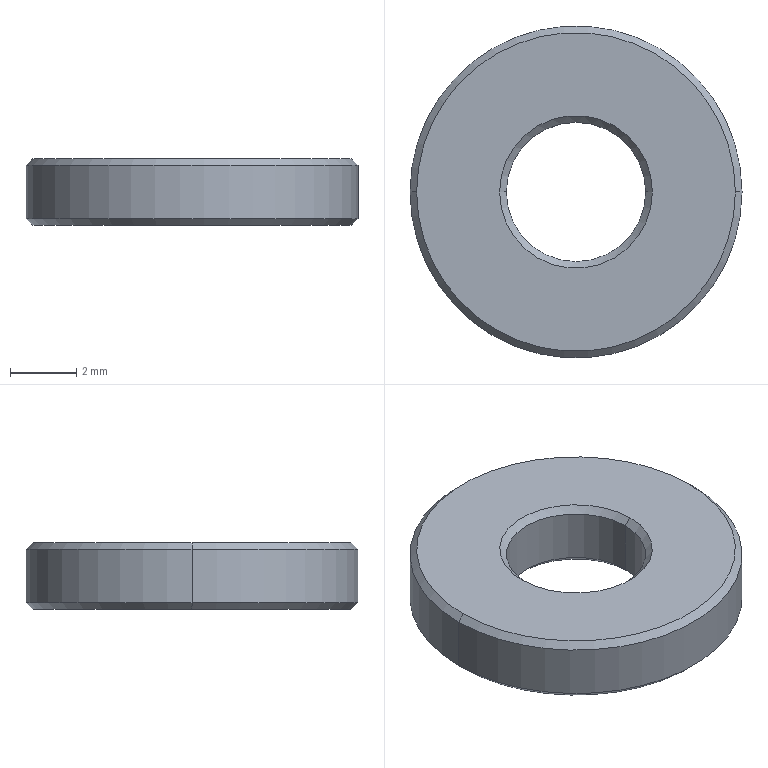Part | NX | features BREP 1 | 1 solid | 14 faces | box 10 x 10 x 2 mm | volume 127.586 mm3 | cone 8 | cylinder 4 | plane 2 | commonest cylinder face diameters 4.2 x2 10 x2
STEP:
#1=CARTESIAN_POINT('',(-4.8,0.,0.));
#2=VERTEX_POINT('',#1);
#3=CARTESIAN_POINT('',(4.8,0.,0.));
#4=VERTEX_POINT('',#3);
#5=CARTESIAN_POINT('',(0.,0.,0.));
#6=DIRECTION('',(0.,0.,-1.));
#7=DIRECTION('',(1.,0.,0.));
#8=AXIS2_PLACEMENT_3D('',#5,#6,#7);
#9=CIRCLE('',#8,4.8);
#10=EDGE_CURVE('',#2,#4,#9,.T.);
#11=ORIENTED_EDGE('',*,*,#10,.F.);
#12=CARTESIAN_POINT('',(-5.,0.,0.2));
#13=VERTEX_POINT('',#12);
#14=CARTESIAN_POINT('',(-5.,0.,0.2));
#15=DIRECTION('',(-0.7071,0.,0.7071));
#16=VECTOR('',#15,1000.);
#17=LINE('',#14,#16);
#18=EDGE_CURVE('',#13,#2,#17,.F.);
#19=ORIENTED_EDGE('',*,*,#18,.F.);
#20=CARTESIAN_POINT('',(5.,0.,0.2));
#21=VERTEX_POINT('',#20);
#22=CARTESIAN_POINT('',(0.,0.,0.2));
#23=DIRECTION('',(0.,0.,1.));
#24=DIRECTION('',(1.,0.,0.));
#25=AXIS2_PLACEMENT_3D('',#22,#23,#24);
#26=CIRCLE('',#25,5.);
#27=EDGE_CURVE('',#21,#13,#26,.T.);
#28=ORIENTED_EDGE('',*,*,#27,.F.);
#29=CARTESIAN_POINT('',(5.,0.,0.2));
#30=DIRECTION('',(0.7071,0.,0.7071));
#31=VECTOR('',#30,1000.);
#32=LINE('',#29,#31);
#33=EDGE_CURVE('',#21,#4,#32,.F.);
#34=ORIENTED_EDGE('',*,*,#33,.T.);
#35=EDGE_LOOP('',(#11,#19,#28,#34));
#36=FACE_BOUND('',#35,.T.);
#37=CARTESIAN_POINT('',(0.,0.,0.2));
#38=DIRECTION('',(0.,0.,1.));
#39=DIRECTION('',(1.,0.,0.));
#40=AXIS2_PLACEMENT_3D('',#37,#38,#39);
#41=CONICAL_SURFACE('',#40,5.,0.7854);
#42=ADVANCED_FACE('',(#36),#41,.T.);
#43=CARTESIAN_POINT('',(4.8,0.,2.));
#44=VERTEX_POINT('',#43);
#45=CARTESIAN_POINT('',(-4.8,0.,2.));
#46=VERTEX_POINT('',#45);
#47=CARTESIAN_POINT('',(0.,0.,2.));
#48=DIRECTION('',(0.,0.,1.));
#49=DIRECTION('',(1.,0.,0.));
#50=AXIS2_PLACEMENT_3D('',#47,#48,#49);
#51=CIRCLE('',#50,4.8);
#52=EDGE_CURVE('',#44,#46,#51,.T.);
#53=ORIENTED_EDGE('',*,*,#52,.F.);
#54=CARTESIAN_POINT('',(5.,0.,1.8));
#55=VERTEX_POINT('',#54);
#56=CARTESIAN_POINT('',(4.8,0.,2.));
#57=DIRECTION('',(0.7071,0.,-0.7071));
#58=VECTOR('',#57,1000.);
#59=LINE('',#56,#58);
#60=EDGE_CURVE('',#44,#55,#59,.T.);
#61=ORIENTED_EDGE('',*,*,#60,.T.);
#62=CARTESIAN_POINT('',(-5.,0.,1.8));
#63=VERTEX_POINT('',#62);
#64=CARTESIAN_POINT('',(0.,0.,1.8));
#65=DIRECTION('',(0.,0.,-1.));
#66=DIRECTION('',(1.,0.,0.));
#67=AXIS2_PLACEMENT_3D('',#64,#65,#66);
#68=CIRCLE('',#67,5.);
#69=EDGE_CURVE('',#63,#55,#68,.T.);
#70=ORIENTED_EDGE('',*,*,#69,.F.);
#71=CARTESIAN_POINT('',(-4.8,0.,2.));
#72=DIRECTION('',(-0.7071,0.,-0.7071));
#73=VECTOR('',#72,1000.);
#74=LINE('',#71,#73);
#75=EDGE_CURVE('',#46,#63,#74,.T.);
#76=ORIENTED_EDGE('',*,*,#75,.F.);
#77=EDGE_LOOP('',(#53,#61,#70,#76));
#78=FACE_BOUND('',#77,.T.);
#79=CARTESIAN_POINT('',(0.,0.,2.));
#80=DIRECTION('',(0.,0.,-1.));
#81=DIRECTION('',(-1.,0.,0.));
#82=AXIS2_PLACEMENT_3D('',#79,#80,#81);
#83=CONICAL_SURFACE('',#82,4.8,0.7854);
#84=ADVANCED_FACE('',(#78),#83,.T.);
#85=CARTESIAN_POINT('',(2.1,0.,0.2));
#86=VERTEX_POINT('',#85);
#87=CARTESIAN_POINT('',(-2.1,0.,0.2));
#88=VERTEX_POINT('',#87);
#89=CARTESIAN_POINT('',(0.,0.,0.2));
#90=DIRECTION('',(0.,0.,-1.));
#91=DIRECTION('',(1.,0.,0.));
#92=AXIS2_PLACEMENT_3D('',#89,#90,#91);
#93=CIRCLE('',#92,2.1);
#94=EDGE_CURVE('',#86,#88,#93,.T.);
#95=ORIENTED_EDGE('',*,*,#94,.F.);
#96=CARTESIAN_POINT('',(2.3,0.,0.));
#97=VERTEX_POINT('',#96);
#98=CARTESIAN_POINT('',(2.3,0.,0.));
#99=DIRECTION('',(0.7071,0.,-0.7071));
#100=VECTOR('',#99,1000.);
#101=LINE('',#98,#100);
#102=EDGE_CURVE('',#86,#97,#101,.T.);
#103=ORIENTED_EDGE('',*,*,#102,.T.);
#104=CARTESIAN_POINT('',(-2.3,0.,0.));
#105=VERTEX_POINT('',#104);
#106=CARTESIAN_POINT('',(0.,0.,0.));
#107=DIRECTION('',(0.,0.,1.));
#108=DIRECTION('',(1.,0.,0.));
#109=AXIS2_PLACEMENT_3D('',#106,#107,#108);
#110=CIRCLE('',#109,2.3);
#111=EDGE_CURVE('',#105,#97,#110,.T.);
#112=ORIENTED_EDGE('',*,*,#111,.F.);
#113=CARTESIAN_POINT('',(-2.3,0.,0.));
#114=DIRECTION('',(-0.7071,0.,-0.7071));
#115=VECTOR('',#114,1000.);
#116=LINE('',#113,#115);
#117=EDGE_CURVE('',#88,#105,#116,.T.);
#118=ORIENTED_EDGE('',*,*,#117,.F.);
#119=EDGE_LOOP('',(#95,#103,#112,#118));
#120=FACE_BOUND('',#119,.T.);
#121=CARTESIAN_POINT('',(0.,0.,0.));
#122=DIRECTION('',(0.,0.,-1.));
#123=DIRECTION('',(-1.,0.,0.));
#124=AXIS2_PLACEMENT_3D('',#121,#122,#123);
#125=CONICAL_SURFACE('',#124,2.3,0.7854);
#126=ADVANCED_FACE('',(#120),#125,.F.);
#127=CARTESIAN_POINT('',(-2.1,0.,1.8));
#128=VERTEX_POINT('',#127);
#129=CARTESIAN_POINT('',(2.1,0.,1.8));
#130=VERTEX_POINT('',#129);
#131=CARTESIAN_POINT('',(0.,0.,1.8));
#132=DIRECTION('',(0.,0.,1.));
#133=DIRECTION('',(1.,0.,0.));
#134=AXIS2_PLACEMENT_3D('',#131,#132,#133);
#135=CIRCLE('',#134,2.1);
#136=EDGE_CURVE('',#128,#130,#135,.T.);
#137=ORIENTED_EDGE('',*,*,#136,.F.);
#138=CARTESIAN_POINT('',(-2.3,0.,2.));
#139=VERTEX_POINT('',#138);
#140=CARTESIAN_POINT('',(-2.1,0.,1.8));
#141=DIRECTION('',(-0.7071,0.,0.7071));
#142=VECTOR('',#141,1000.);
#143=LINE('',#140,#142);
#144=EDGE_CURVE('',#139,#128,#143,.F.);
#145=ORIENTED_EDGE('',*,*,#144,.F.);
#146=CARTESIAN_POINT('',(2.3,0.,2.));
#147=VERTEX_POINT('',#146);
#148=CARTESIAN_POINT('',(0.,0.,2.));
#149=DIRECTION('',(0.,0.,-1.));
#150=DIRECTION('',(1.,0.,0.));
#151=AXIS2_PLACEMENT_3D('',#148,#149,#150);
#152=CIRCLE('',#151,2.3);
#153=EDGE_CURVE('',#147,#139,#152,.T.);
#154=ORIENTED_EDGE('',*,*,#153,.F.);
#155=CARTESIAN_POINT('',(2.1,0.,1.8));
#156=DIRECTION('',(0.7071,0.,0.7071));
#157=VECTOR('',#156,1000.);
#158=LINE('',#155,#157);
#159=EDGE_CURVE('',#147,#130,#158,.F.);
#160=ORIENTED_EDGE('',*,*,#159,.T.);
#161=EDGE_LOOP('',(#137,#145,#154,#160));
#162=FACE_BOUND('',#161,.T.);
#163=CARTESIAN_POINT('',(0.,0.,1.8));
#164=DIRECTION('',(0.,0.,1.));
#165=DIRECTION('',(1.,0.,0.));
#166=AXIS2_PLACEMENT_3D('',#163,#164,#165);
#167=CONICAL_SURFACE('',#166,2.1,0.7854);
#168=ADVANCED_FACE('',(#162),#167,.F.);
#169=ORIENTED_EDGE('',*,*,#136,.T.);
#170=CARTESIAN_POINT('',(2.1,0.,2.));
#171=DIRECTION('',(0.,0.,-1.));
#172=VECTOR('',#171,1000.);
#173=LINE('',#170,#172);
#174=EDGE_CURVE('',#130,#86,#173,.T.);
#175=ORIENTED_EDGE('',*,*,#174,.T.);
#176=ORIENTED_EDGE('',*,*,#94,.T.);
#177=CARTESIAN_POINT('',(-2.1,0.,2.));
#178=DIRECTION('',(0.,0.,-1.));
#179=VECTOR('',#178,1000.);
#180=LINE('',#177,#179);
#181=EDGE_CURVE('',#128,#88,#180,.T.);
#182=ORIENTED_EDGE('',*,*,#181,.F.);
#183=EDGE_LOOP('',(#169,#175,#176,#182));
#184=FACE_BOUND('',#183,.T.);
#185=CARTESIAN_POINT('',(0.,0.,2.));
#186=DIRECTION('',(0.,0.,-1.));
#187=DIRECTION('',(-1.,0.,0.));
#188=AXIS2_PLACEMENT_3D('',#185,#186,#187);
#189=CYLINDRICAL_SURFACE('',#188,2.1);
#190=ADVANCED_FACE('',(#184),#189,.F.);
#191=ORIENTED_EDGE('',*,*,#69,.T.);
#192=CARTESIAN_POINT('',(5.,0.,2.));
#193=DIRECTION('',(0.,0.,-1.));
#194=VECTOR('',#193,1000.);
#195=LINE('',#192,#194);
#196=EDGE_CURVE('',#55,#21,#195,.T.);
#197=ORIENTED_EDGE('',*,*,#196,.T.);
#198=ORIENTED_EDGE('',*,*,#27,.T.);
#199=CARTESIAN_POINT('',(-5.,0.,2.));
#200=DIRECTION('',(0.,0.,-1.));
#201=VECTOR('',#200,1000.);
#202=LINE('',#199,#201);
#203=EDGE_CURVE('',#63,#13,#202,.T.);
#204=ORIENTED_EDGE('',*,*,#203,.F.);
#205=EDGE_LOOP('',(#191,#197,#198,#204));
#206=FACE_BOUND('',#205,.T.);
#207=CARTESIAN_POINT('',(0.,0.,2.));
#208=DIRECTION('',(0.,0.,-1.));
#209=DIRECTION('',(-1.,0.,0.));
#210=AXIS2_PLACEMENT_3D('',#207,#208,#209);
#211=CYLINDRICAL_SURFACE('',#210,5.);
#212=ADVANCED_FACE('',(#206),#211,.T.);
#213=CARTESIAN_POINT('',(0.,0.,2.));
#214=DIRECTION('',(0.,0.,1.));
#215=DIRECTION('',(1.,0.,0.));
#216=AXIS2_PLACEMENT_3D('',#213,#214,#215);
#217=CIRCLE('',#216,4.8);
#218=EDGE_CURVE('',#46,#44,#217,.T.);
#219=ORIENTED_EDGE('',*,*,#218,.T.);
#220=ORIENTED_EDGE('',*,*,#52,.T.);
#221=EDGE_LOOP('',(#219,#220));
#222=FACE_BOUND('',#221,.T.);
#223=ORIENTED_EDGE('',*,*,#153,.T.);
#224=CARTESIAN_POINT('',(0.,0.,2.));
#225=DIRECTION('',(0.,0.,-1.));
#226=DIRECTION('',(1.,0.,0.));
#227=AXIS2_PLACEMENT_3D('',#224,#225,#226);
#228=CIRCLE('',#227,2.3);
#229=EDGE_CURVE('',#139,#147,#228,.T.);
#230=ORIENTED_EDGE('',*,*,#229,.T.);
#231=EDGE_LOOP('',(#223,#230));
#232=FACE_BOUND('',#231,.T.);
#233=CARTESIAN_POINT('',(0.,0.,2.));
#234=DIRECTION('',(0.,0.,1.));
#235=DIRECTION('',(0.,-1.,0.));
#236=AXIS2_PLACEMENT_3D('',#233,#234,#235);
#237=PLANE('',#236);
#238=ADVANCED_FACE('',(#222,#232),#237,.T.);
#239=CARTESIAN_POINT('',(0.,0.,0.));
#240=DIRECTION('',(0.,0.,-1.));
#241=DIRECTION('',(1.,0.,0.));
#242=AXIS2_PLACEMENT_3D('',#239,#240,#241);
#243=CIRCLE('',#242,4.8);
#244=EDGE_CURVE('',#4,#2,#243,.T.);
#245=ORIENTED_EDGE('',*,*,#244,.T.);
#246=ORIENTED_EDGE('',*,*,#10,.T.);
#247=EDGE_LOOP('',(#245,#246));
#248=FACE_BOUND('',#247,.T.);
#249=ORIENTED_EDGE('',*,*,#111,.T.);
#250=CARTESIAN_POINT('',(0.,0.,0.));
#251=DIRECTION('',(0.,0.,1.));
#252=DIRECTION('',(1.,0.,0.));
#253=AXIS2_PLACEMENT_3D('',#250,#251,#252);
#254=CIRCLE('',#253,2.3);
#255=EDGE_CURVE('',#97,#105,#254,.T.);
#256=ORIENTED_EDGE('',*,*,#255,.T.);
#257=EDGE_LOOP('',(#249,#256));
#258=FACE_BOUND('',#257,.T.);
#259=CARTESIAN_POINT('',(0.,0.,0.));
#260=DIRECTION('',(0.,0.,1.));
#261=DIRECTION('',(0.,-1.,0.));
#262=AXIS2_PLACEMENT_3D('',#259,#260,#261);
#263=PLANE('',#262);
#264=ADVANCED_FACE('',(#248,#258),#263,.F.);
#265=ORIENTED_EDGE('',*,*,#196,.F.);
#266=CARTESIAN_POINT('',(0.,0.,1.8));
#267=DIRECTION('',(0.,0.,-1.));
#268=DIRECTION('',(1.,0.,0.));
#269=AXIS2_PLACEMENT_3D('',#266,#267,#268);
#270=CIRCLE('',#269,5.);
#271=EDGE_CURVE('',#55,#63,#270,.T.);
#272=ORIENTED_EDGE('',*,*,#271,.T.);
#273=ORIENTED_EDGE('',*,*,#203,.T.);
#274=CARTESIAN_POINT('',(0.,0.,0.2));
#275=DIRECTION('',(0.,0.,1.));
#276=DIRECTION('',(1.,0.,0.));
#277=AXIS2_PLACEMENT_3D('',#274,#275,#276);
#278=CIRCLE('',#277,5.);
#279=EDGE_CURVE('',#13,#21,#278,.T.);
#280=ORIENTED_EDGE('',*,*,#279,.T.);
#281=EDGE_LOOP('',(#265,#272,#273,#280));
#282=FACE_BOUND('',#281,.T.);
#283=CARTESIAN_POINT('',(0.,0.,2.));
#284=DIRECTION('',(0.,0.,-1.));
#285=DIRECTION('',(-1.,0.,0.));
#286=AXIS2_PLACEMENT_3D('',#283,#284,#285);
#287=CYLINDRICAL_SURFACE('',#286,5.);
#288=ADVANCED_FACE('',(#282),#287,.T.);
#289=ORIENTED_EDGE('',*,*,#174,.F.);
#290=CARTESIAN_POINT('',(0.,0.,1.8));
#291=DIRECTION('',(0.,0.,1.));
#292=DIRECTION('',(1.,0.,0.));
#293=AXIS2_PLACEMENT_3D('',#290,#291,#292);
#294=CIRCLE('',#293,2.1);
#295=EDGE_CURVE('',#130,#128,#294,.T.);
#296=ORIENTED_EDGE('',*,*,#295,.T.);
#297=ORIENTED_EDGE('',*,*,#181,.T.);
#298=CARTESIAN_POINT('',(0.,0.,0.2));
#299=DIRECTION('',(0.,0.,-1.));
#300=DIRECTION('',(1.,0.,0.));
#301=AXIS2_PLACEMENT_3D('',#298,#299,#300);
#302=CIRCLE('',#301,2.1);
#303=EDGE_CURVE('',#88,#86,#302,.T.);
#304=ORIENTED_EDGE('',*,*,#303,.T.);
#305=EDGE_LOOP('',(#289,#296,#297,#304));
#306=FACE_BOUND('',#305,.T.);
#307=CARTESIAN_POINT('',(0.,0.,2.));
#308=DIRECTION('',(0.,0.,-1.));
#309=DIRECTION('',(-1.,0.,0.));
#310=AXIS2_PLACEMENT_3D('',#307,#308,#309);
#311=CYLINDRICAL_SURFACE('',#310,2.1);
#312=ADVANCED_FACE('',(#306),#311,.F.);
#313=ORIENTED_EDGE('',*,*,#144,.T.);
#314=ORIENTED_EDGE('',*,*,#295,.F.);
#315=ORIENTED_EDGE('',*,*,#159,.F.);
#316=ORIENTED_EDGE('',*,*,#229,.F.);
#317=EDGE_LOOP('',(#313,#314,#315,#316));
#318=FACE_BOUND('',#317,.T.);
#319=CARTESIAN_POINT('',(0.,0.,1.8));
#320=DIRECTION('',(0.,0.,1.));
#321=DIRECTION('',(1.,0.,0.));
#322=AXIS2_PLACEMENT_3D('',#319,#320,#321);
#323=CONICAL_SURFACE('',#322,2.1,0.7854);
#324=ADVANCED_FACE('',(#318),#323,.F.);
#325=ORIENTED_EDGE('',*,*,#102,.F.);
#326=ORIENTED_EDGE('',*,*,#303,.F.);
#327=ORIENTED_EDGE('',*,*,#117,.T.);
#328=ORIENTED_EDGE('',*,*,#255,.F.);
#329=EDGE_LOOP('',(#325,#326,#327,#328));
#330=FACE_BOUND('',#329,.T.);
#331=CARTESIAN_POINT('',(0.,0.,0.));
#332=DIRECTION('',(0.,0.,-1.));
#333=DIRECTION('',(-1.,0.,0.));
#334=AXIS2_PLACEMENT_3D('',#331,#332,#333);
#335=CONICAL_SURFACE('',#334,2.3,0.7854);
#336=ADVANCED_FACE('',(#330),#335,.F.);
#337=ORIENTED_EDGE('',*,*,#60,.F.);
#338=ORIENTED_EDGE('',*,*,#218,.F.);
#339=ORIENTED_EDGE('',*,*,#75,.T.);
#340=ORIENTED_EDGE('',*,*,#271,.F.);
#341=EDGE_LOOP('',(#337,#338,#339,#340));
#342=FACE_BOUND('',#341,.T.);
#343=CARTESIAN_POINT('',(0.,0.,2.));
#344=DIRECTION('',(0.,0.,-1.));
#345=DIRECTION('',(-1.,0.,0.));
#346=AXIS2_PLACEMENT_3D('',#343,#344,#345);
#347=CONICAL_SURFACE('',#346,4.8,0.7854);
#348=ADVANCED_FACE('',(#342),#347,.T.);
#349=ORIENTED_EDGE('',*,*,#18,.T.);
#350=ORIENTED_EDGE('',*,*,#244,.F.);
#351=ORIENTED_EDGE('',*,*,#33,.F.);
#352=ORIENTED_EDGE('',*,*,#279,.F.);
#353=EDGE_LOOP('',(#349,#350,#351,#352));
#354=FACE_BOUND('',#353,.T.);
#355=CARTESIAN_POINT('',(0.,0.,0.2));
#356=DIRECTION('',(0.,0.,1.));
#357=DIRECTION('',(1.,0.,0.));
#358=AXIS2_PLACEMENT_3D('',#355,#356,#357);
#359=CONICAL_SURFACE('',#358,5.,0.7854);
#360=ADVANCED_FACE('',(#354),#359,.T.);
#361=CLOSED_SHELL('',(#42,#84,#126,#168,#190,#212,#238,#264,#288,#312,#324,#336,#348,#360));
#362=MANIFOLD_SOLID_BREP('',#361);
#363=(LENGTH_UNIT()NAMED_UNIT(*)SI_UNIT(.MILLI.,.METRE.));
#364=UNCERTAINTY_MEASURE_WITH_UNIT(LENGTH_MEASURE(0.00001),#363,'','');
#365=(NAMED_UNIT(*)PLANE_ANGLE_UNIT()SI_UNIT($,.RADIAN.));
#366=(NAMED_UNIT(*)SI_UNIT($,.STERADIAN.)SOLID_ANGLE_UNIT());
#367=(GEOMETRIC_REPRESENTATION_CONTEXT(3)GLOBAL_UNCERTAINTY_ASSIGNED_CONTEXT((#364))GLOBAL_UNIT_ASSIGNED_CONTEXT((#363,#365,#366))REPRESENTATION_CONTEXT('',''));
#368=ADVANCED_BREP_SHAPE_REPRESENTATION('',(#362),#367);